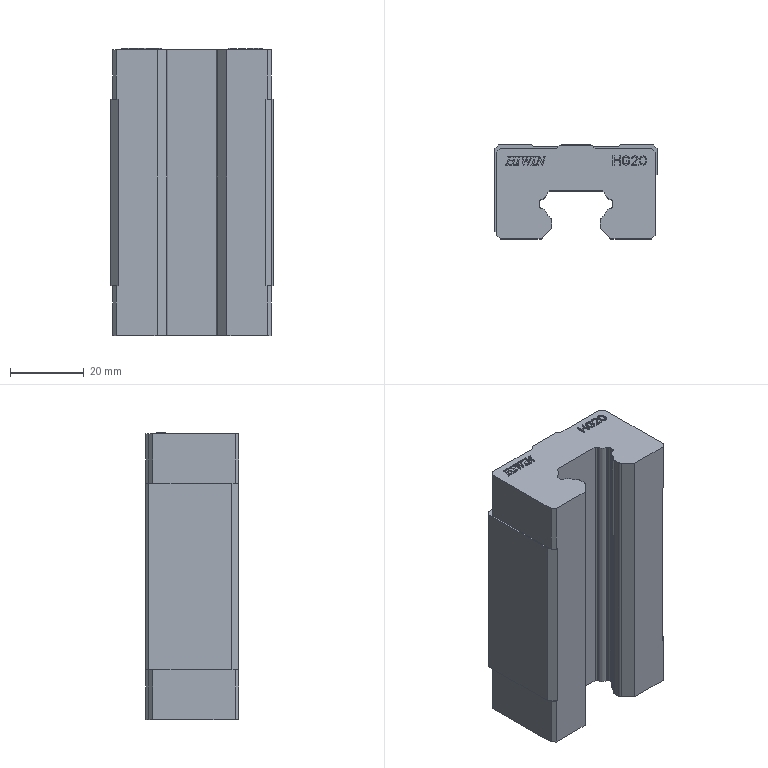Part | NX | 1 solid | 373 faces | box 44 x 25.4 x 77.8 mm | volume 67305 mm3 | plane 285 | spline 60 | cylinder 28 | commonest cylinder face diameters 1 x12 2 x8 4.06 x4 5 x4